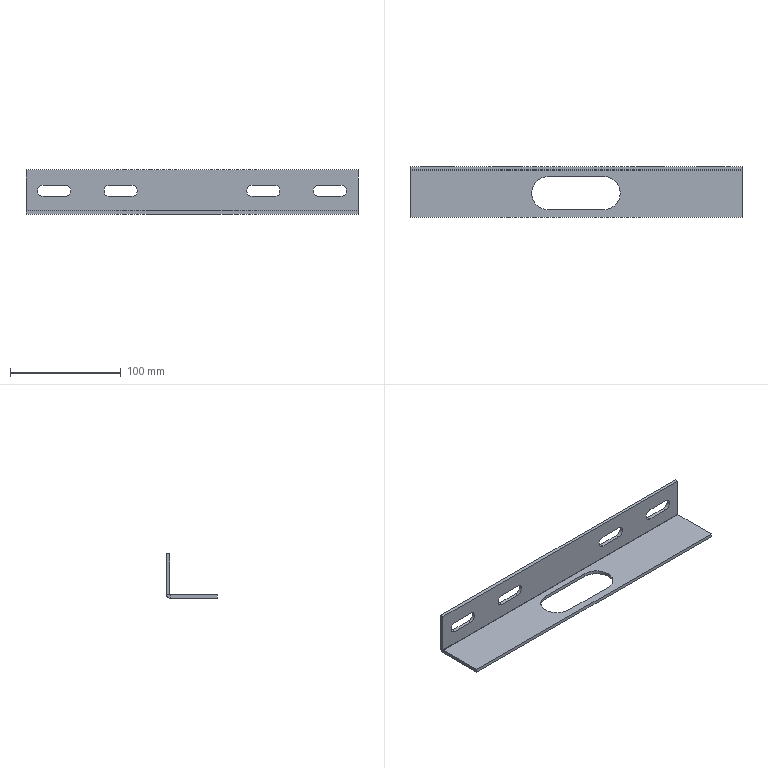Part | 1 solid | 35 faces | box 300 x 46 x 40 mm | volume 64080 mm3 | plane 22 | cylinder 13 | commonest cylinder face diameters 10 x8 30 x3 0.4 x1 6.4 x1
STEP:
#1=CARTESIAN_POINT('',(40.,-1.,-3.));
#2=VERTEX_POINT('',#1);
#3=CARTESIAN_POINT('',(25.,14.,-3.));
#4=VERTEX_POINT('',#3);
#5=CARTESIAN_POINT('',(25.,-1.,-3.));
#6=DIRECTION('',(0.,0.,1.));
#7=DIRECTION('',(1.,0.,0.));
#8=AXIS2_PLACEMENT_3D('',#5,#6,#7);
#9=CIRCLE('',#8,15.);
#10=EDGE_CURVE('',#2,#4,#9,.T.);
#11=ORIENTED_EDGE('',*,*,#10,.F.);
#12=CARTESIAN_POINT('',(40.,-1.,0.));
#13=VERTEX_POINT('',#12);
#14=CARTESIAN_POINT('',(40.,-1.,-10.));
#15=DIRECTION('',(0.,0.,1.));
#16=VECTOR('',#15,1000.);
#17=LINE('',#14,#16);
#18=EDGE_CURVE('',#2,#13,#17,.T.);
#19=ORIENTED_EDGE('',*,*,#18,.T.);
#20=CARTESIAN_POINT('',(25.,14.,0.));
#21=VERTEX_POINT('',#20);
#22=CARTESIAN_POINT('',(25.,-1.,0.));
#23=DIRECTION('',(0.,0.,1.));
#24=DIRECTION('',(1.,0.,0.));
#25=AXIS2_PLACEMENT_3D('',#22,#23,#24);
#26=CIRCLE('',#25,15.);
#27=EDGE_CURVE('',#13,#21,#26,.T.);
#28=ORIENTED_EDGE('',*,*,#27,.T.);
#29=CARTESIAN_POINT('',(25.,14.,-10.));
#30=DIRECTION('',(0.,0.,1.));
#31=VECTOR('',#30,1000.);
#32=LINE('',#29,#31);
#33=EDGE_CURVE('',#4,#21,#32,.T.);
#34=ORIENTED_EDGE('',*,*,#33,.F.);
#35=EDGE_LOOP('',(#11,#19,#28,#34));
#36=FACE_OUTER_BOUND('',#35,.T.);
#37=CARTESIAN_POINT('',(25.,-1.,-10.));
#38=DIRECTION('',(0.,0.,1.));
#39=DIRECTION('',(1.,0.,0.));
#40=AXIS2_PLACEMENT_3D('',#37,#38,#39);
#41=CYLINDRICAL_SURFACE('',#40,15.);
#42=ADVANCED_FACE('',(#36),#41,.F.);
#43=CARTESIAN_POINT('',(-150.,19.8,0.));
#44=VERTEX_POINT('',#43);
#45=CARTESIAN_POINT('',(-150.,-23.,0.));
#46=VERTEX_POINT('',#45);
#47=CARTESIAN_POINT('',(-150.,23.,0.));
#48=DIRECTION('',(0.,-1.,0.));
#49=VECTOR('',#48,1000.);
#50=LINE('',#47,#49);
#51=EDGE_CURVE('',#44,#46,#50,.T.);
#52=ORIENTED_EDGE('',*,*,#51,.F.);
#53=CARTESIAN_POINT('',(-150.,19.8,-3.));
#54=VERTEX_POINT('',#53);
#55=CARTESIAN_POINT('',(-150.,19.8,0.));
#56=DIRECTION('',(0.,0.,-1.));
#57=VECTOR('',#56,1000.);
#58=LINE('',#55,#57);
#59=EDGE_CURVE('',#44,#54,#58,.T.);
#60=ORIENTED_EDGE('',*,*,#59,.T.);
#61=CARTESIAN_POINT('',(-150.,-23.,-3.));
#62=VERTEX_POINT('',#61);
#63=CARTESIAN_POINT('',(-150.,23.,-3.));
#64=DIRECTION('',(0.,-1.,0.));
#65=VECTOR('',#64,1000.);
#66=LINE('',#63,#65);
#67=EDGE_CURVE('',#54,#62,#66,.T.);
#68=ORIENTED_EDGE('',*,*,#67,.T.);
#69=CARTESIAN_POINT('',(-150.,-23.,-3.));
#70=DIRECTION('',(0.,0.,1.));
#71=VECTOR('',#70,1000.);
#72=LINE('',#69,#71);
#73=EDGE_CURVE('',#62,#46,#72,.T.);
#74=ORIENTED_EDGE('',*,*,#73,.T.);
#75=EDGE_LOOP('',(#52,#60,#68,#74));
#76=FACE_OUTER_BOUND('',#75,.T.);
#77=CARTESIAN_POINT('',(-150.,23.,-3.));
#78=DIRECTION('',(-1.,0.,0.));
#79=DIRECTION('',(0.,0.,1.));
#80=AXIS2_PLACEMENT_3D('',#77,#78,#79);
#81=PLANE('',#80);
#82=ADVANCED_FACE('',(#76),#81,.T.);
#83=CARTESIAN_POINT('',(-25.,14.,-3.));
#84=VERTEX_POINT('',#83);
#85=CARTESIAN_POINT('',(0.,14.,-3.));
#86=DIRECTION('',(-1.,0.,0.));
#87=VECTOR('',#86,1000.);
#88=LINE('',#85,#87);
#89=EDGE_CURVE('',#4,#84,#88,.T.);
#90=ORIENTED_EDGE('',*,*,#89,.T.);
#91=CARTESIAN_POINT('',(-25.,-16.,-3.));
#92=VERTEX_POINT('',#91);
#93=CARTESIAN_POINT('',(-25.,-1.,-3.));
#94=DIRECTION('',(0.,0.,1.));
#95=DIRECTION('',(1.,0.,0.));
#96=AXIS2_PLACEMENT_3D('',#93,#94,#95);
#97=CIRCLE('',#96,15.);
#98=EDGE_CURVE('',#84,#92,#97,.T.);
#99=ORIENTED_EDGE('',*,*,#98,.T.);
#100=CARTESIAN_POINT('',(25.,-16.,-3.));
#101=VERTEX_POINT('',#100);
#102=CARTESIAN_POINT('',(0.,-16.,-3.));
#103=DIRECTION('',(1.,0.,0.));
#104=VECTOR('',#103,1000.);
#105=LINE('',#102,#104);
#106=EDGE_CURVE('',#92,#101,#105,.T.);
#107=ORIENTED_EDGE('',*,*,#106,.T.);
#108=CARTESIAN_POINT('',(25.,-1.,-3.));
#109=DIRECTION('',(0.,0.,1.));
#110=DIRECTION('',(1.,0.,0.));
#111=AXIS2_PLACEMENT_3D('',#108,#109,#110);
#112=CIRCLE('',#111,15.);
#113=EDGE_CURVE('',#101,#2,#112,.T.);
#114=ORIENTED_EDGE('',*,*,#113,.T.);
#115=ORIENTED_EDGE('',*,*,#10,.T.);
#116=EDGE_LOOP('',(#90,#99,#107,#114,#115));
#117=FACE_BOUND('',#116,.T.);
#118=CARTESIAN_POINT('',(150.,19.8,-3.));
#119=VERTEX_POINT('',#118);
#120=CARTESIAN_POINT('',(-150.,19.8,-3.));
#121=DIRECTION('',(1.,0.,0.));
#122=VECTOR('',#121,1000.);
#123=LINE('',#120,#122);
#124=EDGE_CURVE('',#54,#119,#123,.T.);
#125=ORIENTED_EDGE('',*,*,#124,.T.);
#126=CARTESIAN_POINT('',(150.,-23.,-3.));
#127=VERTEX_POINT('',#126);
#128=CARTESIAN_POINT('',(150.,23.,-3.));
#129=DIRECTION('',(0.,1.,0.));
#130=VECTOR('',#129,1000.);
#131=LINE('',#128,#130);
#132=EDGE_CURVE('',#127,#119,#131,.T.);
#133=ORIENTED_EDGE('',*,*,#132,.F.);
#134=CARTESIAN_POINT('',(-150.,-23.,-3.));
#135=DIRECTION('',(1.,0.,0.));
#136=VECTOR('',#135,1000.);
#137=LINE('',#134,#136);
#138=EDGE_CURVE('',#62,#127,#137,.T.);
#139=ORIENTED_EDGE('',*,*,#138,.F.);
#140=ORIENTED_EDGE('',*,*,#67,.F.);
#141=EDGE_LOOP('',(#125,#133,#139,#140));
#142=FACE_OUTER_BOUND('',#141,.T.);
#143=CARTESIAN_POINT('',(0.,0.,-3.));
#144=DIRECTION('',(0.,0.,1.));
#145=DIRECTION('',(1.,0.,0.));
#146=AXIS2_PLACEMENT_3D('',#143,#144,#145);
#147=PLANE('',#146);
#148=ADVANCED_FACE('',(#117,#142),#147,.F.);
#149=CARTESIAN_POINT('',(-25.,14.,0.));
#150=VERTEX_POINT('',#149);
#151=CARTESIAN_POINT('',(-25.,-16.,0.));
#152=VERTEX_POINT('',#151);
#153=CARTESIAN_POINT('',(-25.,-1.,0.));
#154=DIRECTION('',(0.,0.,1.));
#155=DIRECTION('',(1.,0.,0.));
#156=AXIS2_PLACEMENT_3D('',#153,#154,#155);
#157=CIRCLE('',#156,15.);
#158=EDGE_CURVE('',#150,#152,#157,.T.);
#159=ORIENTED_EDGE('',*,*,#158,.F.);
#160=CARTESIAN_POINT('',(-25.,14.,0.));
#161=DIRECTION('',(-1.,0.,0.));
#162=VECTOR('',#161,1000.);
#163=LINE('',#160,#162);
#164=EDGE_CURVE('',#21,#150,#163,.T.);
#165=ORIENTED_EDGE('',*,*,#164,.F.);
#166=ORIENTED_EDGE('',*,*,#27,.F.);
#167=CARTESIAN_POINT('',(25.,-16.,0.));
#168=VERTEX_POINT('',#167);
#169=CARTESIAN_POINT('',(25.,-1.,0.));
#170=DIRECTION('',(0.,0.,1.));
#171=DIRECTION('',(1.,0.,0.));
#172=AXIS2_PLACEMENT_3D('',#169,#170,#171);
#173=CIRCLE('',#172,15.);
#174=EDGE_CURVE('',#168,#13,#173,.T.);
#175=ORIENTED_EDGE('',*,*,#174,.F.);
#176=CARTESIAN_POINT('',(-25.,-16.,0.));
#177=DIRECTION('',(1.,0.,0.));
#178=VECTOR('',#177,1000.);
#179=LINE('',#176,#178);
#180=EDGE_CURVE('',#152,#168,#179,.T.);
#181=ORIENTED_EDGE('',*,*,#180,.F.);
#182=EDGE_LOOP('',(#159,#165,#166,#175,#181));
#183=FACE_BOUND('',#182,.T.);
#184=CARTESIAN_POINT('',(150.,-23.,0.));
#185=VERTEX_POINT('',#184);
#186=CARTESIAN_POINT('',(150.,19.8,0.));
#187=VERTEX_POINT('',#186);
#188=CARTESIAN_POINT('',(150.,23.,0.));
#189=DIRECTION('',(0.,1.,0.));
#190=VECTOR('',#189,1000.);
#191=LINE('',#188,#190);
#192=EDGE_CURVE('',#185,#187,#191,.T.);
#193=ORIENTED_EDGE('',*,*,#192,.T.);
#194=CARTESIAN_POINT('',(-150.,19.8,0.));
#195=DIRECTION('',(1.,0.,0.));
#196=VECTOR('',#195,1000.);
#197=LINE('',#194,#196);
#198=EDGE_CURVE('',#44,#187,#197,.T.);
#199=ORIENTED_EDGE('',*,*,#198,.F.);
#200=ORIENTED_EDGE('',*,*,#51,.T.);
#201=CARTESIAN_POINT('',(-150.,-23.,0.));
#202=DIRECTION('',(1.,0.,0.));
#203=VECTOR('',#202,1000.);
#204=LINE('',#201,#203);
#205=EDGE_CURVE('',#46,#185,#204,.T.);
#206=ORIENTED_EDGE('',*,*,#205,.T.);
#207=EDGE_LOOP('',(#193,#199,#200,#206));
#208=FACE_OUTER_BOUND('',#207,.T.);
#209=CARTESIAN_POINT('',(0.,0.,0.));
#210=DIRECTION('',(0.,0.,1.));
#211=DIRECTION('',(1.,0.,0.));
#212=AXIS2_PLACEMENT_3D('',#209,#210,#211);
#213=PLANE('',#212);
#214=ADVANCED_FACE('',(#183,#208),#213,.T.);
#215=CARTESIAN_POINT('',(150.,19.8,0.));
#216=DIRECTION('',(0.,0.,-1.));
#217=VECTOR('',#216,1000.);
#218=LINE('',#215,#217);
#219=EDGE_CURVE('',#187,#119,#218,.T.);
#220=ORIENTED_EDGE('',*,*,#219,.F.);
#221=ORIENTED_EDGE('',*,*,#192,.F.);
#222=CARTESIAN_POINT('',(150.,-23.,-3.));
#223=DIRECTION('',(0.,0.,1.));
#224=VECTOR('',#223,1000.);
#225=LINE('',#222,#224);
#226=EDGE_CURVE('',#127,#185,#225,.T.);
#227=ORIENTED_EDGE('',*,*,#226,.F.);
#228=ORIENTED_EDGE('',*,*,#132,.T.);
#229=EDGE_LOOP('',(#220,#221,#227,#228));
#230=FACE_OUTER_BOUND('',#229,.T.);
#231=CARTESIAN_POINT('',(150.,23.,-3.));
#232=DIRECTION('',(1.,0.,0.));
#233=DIRECTION('',(0.,0.,-1.));
#234=AXIS2_PLACEMENT_3D('',#231,#232,#233);
#235=PLANE('',#234);
#236=ADVANCED_FACE('',(#230),#235,.T.);
#237=ORIENTED_EDGE('',*,*,#205,.F.);
#238=ORIENTED_EDGE('',*,*,#73,.F.);
#239=ORIENTED_EDGE('',*,*,#138,.T.);
#240=ORIENTED_EDGE('',*,*,#226,.T.);
#241=EDGE_LOOP('',(#237,#238,#239,#240));
#242=FACE_OUTER_BOUND('',#241,.T.);
#243=CARTESIAN_POINT('',(-150.,-23.,-3.));
#244=DIRECTION('',(0.,-1.,0.));
#245=DIRECTION('',(0.,0.,-1.));
#246=AXIS2_PLACEMENT_3D('',#243,#244,#245);
#247=PLANE('',#246);
#248=ADVANCED_FACE('',(#242),#247,.T.);
#249=CARTESIAN_POINT('',(150.,20.,0.2));
#250=VERTEX_POINT('',#249);
#251=CARTESIAN_POINT('',(150.,23.,0.2));
#252=VERTEX_POINT('',#251);
#253=CARTESIAN_POINT('',(150.,23.,0.2));
#254=DIRECTION('',(0.,1.,0.));
#255=VECTOR('',#254,1000.);
#256=LINE('',#253,#255);
#257=EDGE_CURVE('',#250,#252,#256,.T.);
#258=ORIENTED_EDGE('',*,*,#257,.F.);
#259=CARTESIAN_POINT('',(150.,19.8,0.2));
#260=DIRECTION('',(1.,0.,0.));
#261=DIRECTION('',(0.,0.,1.));
#262=AXIS2_PLACEMENT_3D('',#259,#260,#261);
#263=CIRCLE('',#262,0.2);
#264=EDGE_CURVE('',#187,#250,#263,.T.);
#265=ORIENTED_EDGE('',*,*,#264,.F.);
#266=ORIENTED_EDGE('',*,*,#219,.T.);
#267=CARTESIAN_POINT('',(150.,19.8,0.2));
#268=DIRECTION('',(1.,0.,0.));
#269=DIRECTION('',(0.,0.,1.));
#270=AXIS2_PLACEMENT_3D('',#267,#268,#269);
#271=CIRCLE('',#270,3.2);
#272=EDGE_CURVE('',#119,#252,#271,.T.);
#273=ORIENTED_EDGE('',*,*,#272,.T.);
#274=EDGE_LOOP('',(#258,#265,#266,#273));
#275=FACE_OUTER_BOUND('',#274,.T.);
#276=CARTESIAN_POINT('',(150.,19.8,0.2));
#277=DIRECTION('',(1.,0.,0.));
#278=DIRECTION('',(0.,0.,-1.));
#279=AXIS2_PLACEMENT_3D('',#276,#277,#278);
#280=PLANE('',#279);
#281=ADVANCED_FACE('',(#275),#280,.T.);
#282=CARTESIAN_POINT('',(-150.,20.,0.2));
#283=VERTEX_POINT('',#282);
#284=CARTESIAN_POINT('',(-150.,19.8,0.2));
#285=DIRECTION('',(-1.,0.,0.));
#286=DIRECTION('',(0.,0.,1.));
#287=AXIS2_PLACEMENT_3D('',#284,#285,#286);
#288=CIRCLE('',#287,0.2);
#289=EDGE_CURVE('',#283,#44,#288,.T.);
#290=ORIENTED_EDGE('',*,*,#289,.F.);
#291=CARTESIAN_POINT('',(-150.,23.,0.2));
#292=VERTEX_POINT('',#291);
#293=CARTESIAN_POINT('',(-150.,20.,0.2));
#294=DIRECTION('',(0.,1.,0.));
#295=VECTOR('',#294,1000.);
#296=LINE('',#293,#295);
#297=EDGE_CURVE('',#283,#292,#296,.T.);
#298=ORIENTED_EDGE('',*,*,#297,.T.);
#299=CARTESIAN_POINT('',(-150.,19.8,0.2));
#300=DIRECTION('',(-1.,0.,0.));
#301=DIRECTION('',(0.,0.,1.));
#302=AXIS2_PLACEMENT_3D('',#299,#300,#301);
#303=CIRCLE('',#302,3.2);
#304=EDGE_CURVE('',#292,#54,#303,.T.);
#305=ORIENTED_EDGE('',*,*,#304,.T.);
#306=ORIENTED_EDGE('',*,*,#59,.F.);
#307=EDGE_LOOP('',(#290,#298,#305,#306));
#308=FACE_OUTER_BOUND('',#307,.T.);
#309=CARTESIAN_POINT('',(-150.,19.8,0.2));
#310=DIRECTION('',(1.,0.,0.));
#311=DIRECTION('',(0.,0.,-1.));
#312=AXIS2_PLACEMENT_3D('',#309,#310,#311);
#313=PLANE('',#312);
#314=ADVANCED_FACE('',(#308),#313,.F.);
#315=ORIENTED_EDGE('',*,*,#124,.F.);
#316=ORIENTED_EDGE('',*,*,#304,.F.);
#317=CARTESIAN_POINT('',(150.,23.,0.2));
#318=DIRECTION('',(1.,0.,0.));
#319=VECTOR('',#318,1000.);
#320=LINE('',#317,#319);
#321=EDGE_CURVE('',#292,#252,#320,.T.);
#322=ORIENTED_EDGE('',*,*,#321,.T.);
#323=ORIENTED_EDGE('',*,*,#272,.F.);
#324=EDGE_LOOP('',(#315,#316,#322,#323));
#325=FACE_OUTER_BOUND('',#324,.T.);
#326=CARTESIAN_POINT('',(-150.,19.8,0.2));
#327=DIRECTION('',(-1.,0.,0.));
#328=DIRECTION('',(0.,1.,0.));
#329=AXIS2_PLACEMENT_3D('',#326,#327,#328);
#330=CYLINDRICAL_SURFACE('',#329,3.2);
#331=ADVANCED_FACE('',(#325),#330,.T.);
#332=ORIENTED_EDGE('',*,*,#198,.T.);
#333=ORIENTED_EDGE('',*,*,#264,.T.);
#334=CARTESIAN_POINT('',(150.,20.,0.2));
#335=DIRECTION('',(-1.,0.,0.));
#336=VECTOR('',#335,1000.);
#337=LINE('',#334,#336);
#338=EDGE_CURVE('',#250,#283,#337,.T.);
#339=ORIENTED_EDGE('',*,*,#338,.T.);
#340=ORIENTED_EDGE('',*,*,#289,.T.);
#341=EDGE_LOOP('',(#332,#333,#339,#340));
#342=FACE_OUTER_BOUND('',#341,.T.);
#343=CARTESIAN_POINT('',(-150.,19.8,0.2));
#344=DIRECTION('',(-1.,0.,0.));
#345=DIRECTION('',(0.,1.,0.));
#346=AXIS2_PLACEMENT_3D('',#343,#344,#345);
#347=CYLINDRICAL_SURFACE('',#346,0.2);
#348=ADVANCED_FACE('',(#342),#347,.F.);
#349=ORIENTED_EDGE('',*,*,#257,.T.);
#350=CARTESIAN_POINT('',(150.,23.,37.));
#351=VERTEX_POINT('',#350);
#352=CARTESIAN_POINT('',(150.,23.,0.));
#353=DIRECTION('',(0.,0.,-1.));
#354=VECTOR('',#353,1000.);
#355=LINE('',#352,#354);
#356=EDGE_CURVE('',#351,#252,#355,.T.);
#357=ORIENTED_EDGE('',*,*,#356,.F.);
#358=CARTESIAN_POINT('',(150.,20.,37.));
#359=VERTEX_POINT('',#358);
#360=CARTESIAN_POINT('',(150.,23.,37.));
#361=DIRECTION('',(0.,-1.,0.));
#362=VECTOR('',#361,1000.);
#363=LINE('',#360,#362);
#364=EDGE_CURVE('',#351,#359,#363,.T.);
#365=ORIENTED_EDGE('',*,*,#364,.T.);
#366=CARTESIAN_POINT('',(150.,20.,0.));
#367=DIRECTION('',(0.,0.,-1.));
#368=VECTOR('',#367,1000.);
#369=LINE('',#366,#368);
#370=EDGE_CURVE('',#359,#250,#369,.T.);
#371=ORIENTED_EDGE('',*,*,#370,.T.);
#372=EDGE_LOOP('',(#349,#357,#365,#371));
#373=FACE_OUTER_BOUND('',#372,.T.);
#374=CARTESIAN_POINT('',(150.,23.,0.));
#375=DIRECTION('',(-1.,0.,0.));
#376=DIRECTION('',(0.,0.,1.));
#377=AXIS2_PLACEMENT_3D('',#374,#375,#376);
#378=PLANE('',#377);
#379=ADVANCED_FACE('',(#373),#378,.F.);
#380=ORIENTED_EDGE('',*,*,#297,.F.);
#381=CARTESIAN_POINT('',(-150.,20.,37.));
#382=VERTEX_POINT('',#381);
#383=CARTESIAN_POINT('',(-150.,20.,37.));
#384=DIRECTION('',(0.,0.,1.));
#385=VECTOR('',#384,1000.);
#386=LINE('',#383,#385);
#387=EDGE_CURVE('',#283,#382,#386,.T.);
#388=ORIENTED_EDGE('',*,*,#387,.T.);
#389=CARTESIAN_POINT('',(-150.,23.,37.));
#390=VERTEX_POINT('',#389);
#391=CARTESIAN_POINT('',(-150.,23.,37.));
#392=DIRECTION('',(0.,-1.,0.));
#393=VECTOR('',#392,1000.);
#394=LINE('',#391,#393);
#395=EDGE_CURVE('',#390,#382,#394,.T.);
#396=ORIENTED_EDGE('',*,*,#395,.F.);
#397=CARTESIAN_POINT('',(-150.,23.,0.));
#398=DIRECTION('',(0.,0.,1.));
#399=VECTOR('',#398,1000.);
#400=LINE('',#397,#399);
#401=EDGE_CURVE('',#292,#390,#400,.T.);
#402=ORIENTED_EDGE('',*,*,#401,.F.);
#403=EDGE_LOOP('',(#380,#388,#396,#402));
#404=FACE_OUTER_BOUND('',#403,.T.);
#405=CARTESIAN_POINT('',(-150.,23.,37.));
#406=DIRECTION('',(1.,0.,0.));
#407=DIRECTION('',(0.,0.,-1.));
#408=AXIS2_PLACEMENT_3D('',#405,#406,#407);
#409=PLANE('',#408);
#410=ADVANCED_FACE('',(#404),#409,.F.);
#411=CARTESIAN_POINT('',(-134.5,23.,23.));
#412=VERTEX_POINT('',#411);
#413=CARTESIAN_POINT('',(-114.5,23.,23.));
#414=VERTEX_POINT('',#413);
#415=CARTESIAN_POINT('',(-134.5,23.,23.));
#416=DIRECTION('',(1.,0.,0.));
#417=VECTOR('',#416,1000.);
#418=LINE('',#415,#417);
#419=EDGE_CURVE('',#412,#414,#418,.T.);
#420=ORIENTED_EDGE('',*,*,#419,.F.);
#421=CARTESIAN_POINT('',(-134.5,23.,13.));
#422=VERTEX_POINT('',#421);
#423=CARTESIAN_POINT('',(-134.5,23.,18.));
#424=DIRECTION('',(0.,1.,0.));
#425=DIRECTION('',(0.,0.,1.));
#426=AXIS2_PLACEMENT_3D('',#423,#424,#425);
#427=CIRCLE('',#426,5.);
#428=EDGE_CURVE('',#422,#412,#427,.T.);
#429=ORIENTED_EDGE('',*,*,#428,.F.);
#430=CARTESIAN_POINT('',(-114.5,23.,13.));
#431=VERTEX_POINT('',#430);
#432=CARTESIAN_POINT('',(-134.5,23.,13.));
#433=DIRECTION('',(-1.,0.,0.));
#434=VECTOR('',#433,1000.);
#435=LINE('',#432,#434);
#436=EDGE_CURVE('',#431,#422,#435,.T.);
#437=ORIENTED_EDGE('',*,*,#436,.F.);
#438=CARTESIAN_POINT('',(-114.5,23.,18.));
#439=DIRECTION('',(0.,1.,0.));
#440=DIRECTION('',(0.,0.,1.));
#441=AXIS2_PLACEMENT_3D('',#438,#439,#440);
#442=CIRCLE('',#441,5.);
#443=EDGE_CURVE('',#414,#431,#442,.T.);
#444=ORIENTED_EDGE('',*,*,#443,.F.);
#445=EDGE_LOOP('',(#420,#429,#437,#444));
#446=FACE_BOUND('',#445,.T.);
#447=CARTESIAN_POINT('',(-74.5,23.,23.));
#448=VERTEX_POINT('',#447);
#449=CARTESIAN_POINT('',(-54.5,23.,23.));
#450=VERTEX_POINT('',#449);
#451=CARTESIAN_POINT('',(-74.5,23.,23.));
#452=DIRECTION('',(1.,0.,0.));
#453=VECTOR('',#452,1000.);
#454=LINE('',#451,#453);
#455=EDGE_CURVE('',#448,#450,#454,.T.);
#456=ORIENTED_EDGE('',*,*,#455,.F.);
#457=CARTESIAN_POINT('',(-74.5,23.,13.));
#458=VERTEX_POINT('',#457);
#459=CARTESIAN_POINT('',(-74.5,23.,18.));
#460=DIRECTION('',(0.,1.,0.));
#461=DIRECTION('',(0.,0.,1.));
#462=AXIS2_PLACEMENT_3D('',#459,#460,#461);
#463=CIRCLE('',#462,5.);
#464=EDGE_CURVE('',#458,#448,#463,.T.);
#465=ORIENTED_EDGE('',*,*,#464,.F.);
#466=CARTESIAN_POINT('',(-54.5,23.,13.));
#467=VERTEX_POINT('',#466);
#468=CARTESIAN_POINT('',(-74.5,23.,13.));
#469=DIRECTION('',(-1.,0.,0.));
#470=VECTOR('',#469,1000.);
#471=LINE('',#468,#470);
#472=EDGE_CURVE('',#467,#458,#471,.T.);
#473=ORIENTED_EDGE('',*,*,#472,.F.);
#474=CARTESIAN_POINT('',(-54.5,23.,18.));
#475=DIRECTION('',(0.,1.,0.));
#476=DIRECTION('',(0.,0.,1.));
#477=AXIS2_PLACEMENT_3D('',#474,#475,#476);
#478=CIRCLE('',#477,5.);
#479=EDGE_CURVE('',#450,#467,#478,.T.);
#480=ORIENTED_EDGE('',*,*,#479,.F.);
#481=EDGE_LOOP('',(#456,#465,#473,#480));
#482=FACE_BOUND('',#481,.T.);
#483=CARTESIAN_POINT('',(74.5,23.,13.));
#484=VERTEX_POINT('',#483);
#485=CARTESIAN_POINT('',(54.5,23.,13.));
#486=VERTEX_POINT('',#485);
#487=CARTESIAN_POINT('',(74.5,23.,13.));
#488=DIRECTION('',(-1.,0.,0.));
#489=VECTOR('',#488,1000.);
#490=LINE('',#487,#489);
#491=EDGE_CURVE('',#484,#486,#490,.T.);
#492=ORIENTED_EDGE('',*,*,#491,.F.);
#493=CARTESIAN_POINT('',(74.5,23.,23.));
#494=VERTEX_POINT('',#493);
#495=CARTESIAN_POINT('',(74.5,23.,18.));
#496=DIRECTION('',(0.,1.,0.));
#497=DIRECTION('',(0.,0.,-1.));
#498=AXIS2_PLACEMENT_3D('',#495,#496,#497);
#499=CIRCLE('',#498,5.);
#500=EDGE_CURVE('',#494,#484,#499,.T.);
#501=ORIENTED_EDGE('',*,*,#500,.F.);
#502=CARTESIAN_POINT('',(54.5,23.,23.));
#503=VERTEX_POINT('',#502);
#504=CARTESIAN_POINT('',(74.5,23.,23.));
#505=DIRECTION('',(1.,0.,0.));
#506=VECTOR('',#505,1000.);
#507=LINE('',#504,#506);
#508=EDGE_CURVE('',#503,#494,#507,.T.);
#509=ORIENTED_EDGE('',*,*,#508,.F.);
#510=CARTESIAN_POINT('',(54.5,23.,18.));
#511=DIRECTION('',(0.,1.,0.));
#512=DIRECTION('',(0.,0.,-1.));
#513=AXIS2_PLACEMENT_3D('',#510,#511,#512);
#514=CIRCLE('',#513,5.);
#515=EDGE_CURVE('',#486,#503,#514,.T.);
#516=ORIENTED_EDGE('',*,*,#515,.F.);
#517=EDGE_LOOP('',(#492,#501,#509,#516));
#518=FACE_BOUND('',#517,.T.);
#519=CARTESIAN_POINT('',(134.5,23.,13.));
#520=VERTEX_POINT('',#519);
#521=CARTESIAN_POINT('',(114.5,23.,13.));
#522=VERTEX_POINT('',#521);
#523=CARTESIAN_POINT('',(134.5,23.,13.));
#524=DIRECTION('',(-1.,0.,0.));
#525=VECTOR('',#524,1000.);
#526=LINE('',#523,#525);
#527=EDGE_CURVE('',#520,#522,#526,.T.);
#528=ORIENTED_EDGE('',*,*,#527,.F.);
#529=CARTESIAN_POINT('',(134.5,23.,23.));
#530=VERTEX_POINT('',#529);
#531=CARTESIAN_POINT('',(134.5,23.,18.));
#532=DIRECTION('',(0.,1.,0.));
#533=DIRECTION('',(0.,0.,-1.));
#534=AXIS2_PLACEMENT_3D('',#531,#532,#533);
#535=CIRCLE('',#534,5.);
#536=EDGE_CURVE('',#530,#520,#535,.T.);
#537=ORIENTED_EDGE('',*,*,#536,.F.);
#538=CARTESIAN_POINT('',(114.5,23.,23.));
#539=VERTEX_POINT('',#538);
#540=CARTESIAN_POINT('',(134.5,23.,23.));
#541=DIRECTION('',(1.,0.,0.));
#542=VECTOR('',#541,1000.);
#543=LINE('',#540,#542);
#544=EDGE_CURVE('',#539,#530,#543,.T.);
#545=ORIENTED_EDGE('',*,*,#544,.F.);
#546=CARTESIAN_POINT('',(114.5,23.,18.));
#547=DIRECTION('',(0.,1.,0.));
#548=DIRECTION('',(0.,0.,-1.));
#549=AXIS2_PLACEMENT_3D('',#546,#547,#548);
#550=CIRCLE('',#549,5.);
#551=EDGE_CURVE('',#522,#539,#550,.T.);
#552=ORIENTED_EDGE('',*,*,#551,.F.);
#553=EDGE_LOOP('',(#528,#537,#545,#552));
#554=FACE_BOUND('',#553,.T.);
#555=ORIENTED_EDGE('',*,*,#321,.F.);
#556=ORIENTED_EDGE('',*,*,#401,.T.);
#557=CARTESIAN_POINT('',(0.,23.,37.));
#558=DIRECTION('',(1.,0.,0.));
#559=VECTOR('',#558,1000.);
#560=LINE('',#557,#559);
#561=EDGE_CURVE('',#390,#351,#560,.T.);
#562=ORIENTED_EDGE('',*,*,#561,.T.);
#563=ORIENTED_EDGE('',*,*,#356,.T.);
#564=EDGE_LOOP('',(#555,#556,#562,#563));
#565=FACE_OUTER_BOUND('',#564,.T.);
#566=CARTESIAN_POINT('',(0.,23.,0.));
#567=DIRECTION('',(0.,-1.,0.));
#568=DIRECTION('',(0.,0.,-1.));
#569=AXIS2_PLACEMENT_3D('',#566,#567,#568);
#570=PLANE('',#569);
#571=ADVANCED_FACE('',(#446,#482,#518,#554,#565),#570,.F.);
#572=CARTESIAN_POINT('',(-134.5,20.,23.));
#573=VERTEX_POINT('',#572);
#574=CARTESIAN_POINT('',(-134.5,20.,13.));
#575=VERTEX_POINT('',#574);
#576=CARTESIAN_POINT('',(-134.5,20.,18.));
#577=DIRECTION('',(0.,-1.,0.));
#578=DIRECTION('',(0.,0.,-1.));
#579=AXIS2_PLACEMENT_3D('',#576,#577,#578);
#580=CIRCLE('',#579,5.);
#581=EDGE_CURVE('',#573,#575,#580,.T.);
#582=ORIENTED_EDGE('',*,*,#581,.F.);
#583=CARTESIAN_POINT('',(-114.5,20.,23.));
#584=VERTEX_POINT('',#583);
#585=CARTESIAN_POINT('',(0.,20.,23.));
#586=DIRECTION('',(-1.,0.,0.));
#587=VECTOR('',#586,1000.);
#588=LINE('',#585,#587);
#589=EDGE_CURVE('',#584,#573,#588,.T.);
#590=ORIENTED_EDGE('',*,*,#589,.F.);
#591=CARTESIAN_POINT('',(-114.5,20.,13.));
#592=VERTEX_POINT('',#591);
#593=CARTESIAN_POINT('',(-114.5,20.,18.));
#594=DIRECTION('',(0.,-1.,0.));
#595=DIRECTION('',(0.,0.,-1.));
#596=AXIS2_PLACEMENT_3D('',#593,#594,#595);
#597=CIRCLE('',#596,5.);
#598=EDGE_CURVE('',#592,#584,#597,.T.);
#599=ORIENTED_EDGE('',*,*,#598,.F.);
#600=CARTESIAN_POINT('',(0.,20.,13.));
#601=DIRECTION('',(1.,0.,0.));
#602=VECTOR('',#601,1000.);
#603=LINE('',#600,#602);
#604=EDGE_CURVE('',#575,#592,#603,.T.);
#605=ORIENTED_EDGE('',*,*,#604,.F.);
#606=EDGE_LOOP('',(#582,#590,#599,#605));
#607=FACE_BOUND('',#606,.T.);
#608=CARTESIAN_POINT('',(-74.5,20.,23.));
#609=VERTEX_POINT('',#608);
#610=CARTESIAN_POINT('',(-74.5,20.,13.));
#611=VERTEX_POINT('',#610);
#612=CARTESIAN_POINT('',(-74.5,20.,18.));
#613=DIRECTION('',(0.,-1.,0.));
#614=DIRECTION('',(0.,0.,-1.));
#615=AXIS2_PLACEMENT_3D('',#612,#613,#614);
#616=CIRCLE('',#615,5.);
#617=EDGE_CURVE('',#609,#611,#616,.T.);
#618=ORIENTED_EDGE('',*,*,#617,.F.);
#619=CARTESIAN_POINT('',(-54.5,20.,23.));
#620=VERTEX_POINT('',#619);
#621=CARTESIAN_POINT('',(0.,20.,23.));
#622=DIRECTION('',(-1.,0.,0.));
#623=VECTOR('',#622,1000.);
#624=LINE('',#621,#623);
#625=EDGE_CURVE('',#620,#609,#624,.T.);
#626=ORIENTED_EDGE('',*,*,#625,.F.);
#627=CARTESIAN_POINT('',(-54.5,20.,13.));
#628=VERTEX_POINT('',#627);
#629=CARTESIAN_POINT('',(-54.5,20.,18.));
#630=DIRECTION('',(0.,-1.,0.));
#631=DIRECTION('',(0.,0.,-1.));
#632=AXIS2_PLACEMENT_3D('',#629,#630,#631);
#633=CIRCLE('',#632,5.);
#634=EDGE_CURVE('',#628,#620,#633,.T.);
#635=ORIENTED_EDGE('',*,*,#634,.F.);
#636=CARTESIAN_POINT('',(0.,20.,13.));
#637=DIRECTION('',(1.,0.,0.));
#638=VECTOR('',#637,1000.);
#639=LINE('',#636,#638);
#640=EDGE_CURVE('',#611,#628,#639,.T.);
#641=ORIENTED_EDGE('',*,*,#640,.F.);
#642=EDGE_LOOP('',(#618,#626,#635,#641));
#643=FACE_BOUND('',#642,.T.);
#644=CARTESIAN_POINT('',(74.5,20.,13.));
#645=VERTEX_POINT('',#644);
#646=CARTESIAN_POINT('',(74.5,20.,23.));
#647=VERTEX_POINT('',#646);
#648=CARTESIAN_POINT('',(74.5,20.,18.));
#649=DIRECTION('',(0.,-1.,0.));
#650=DIRECTION('',(0.,0.,-1.));
#651=AXIS2_PLACEMENT_3D('',#648,#649,#650);
#652=CIRCLE('',#651,5.);
#653=EDGE_CURVE('',#645,#647,#652,.T.);
#654=ORIENTED_EDGE('',*,*,#653,.F.);
#655=CARTESIAN_POINT('',(54.5,20.,13.));
#656=VERTEX_POINT('',#655);
#657=CARTESIAN_POINT('',(0.,20.,13.));
#658=DIRECTION('',(1.,0.,0.));
#659=VECTOR('',#658,1000.);
#660=LINE('',#657,#659);
#661=EDGE_CURVE('',#656,#645,#660,.T.);
#662=ORIENTED_EDGE('',*,*,#661,.F.);
#663=CARTESIAN_POINT('',(54.5,20.,23.));
#664=VERTEX_POINT('',#663);
#665=CARTESIAN_POINT('',(54.5,20.,18.));
#666=DIRECTION('',(0.,-1.,0.));
#667=DIRECTION('',(0.,0.,-1.));
#668=AXIS2_PLACEMENT_3D('',#665,#666,#667);
#669=CIRCLE('',#668,5.);
#670=EDGE_CURVE('',#664,#656,#669,.T.);
#671=ORIENTED_EDGE('',*,*,#670,.F.);
#672=CARTESIAN_POINT('',(0.,20.,23.));
#673=DIRECTION('',(-1.,0.,0.));
#674=VECTOR('',#673,1000.);
#675=LINE('',#672,#674);
#676=EDGE_CURVE('',#647,#664,#675,.T.);
#677=ORIENTED_EDGE('',*,*,#676,.F.);
#678=EDGE_LOOP('',(#654,#662,#671,#677));
#679=FACE_BOUND('',#678,.T.);
#680=CARTESIAN_POINT('',(134.5,20.,13.));
#681=VERTEX_POINT('',#680);
#682=CARTESIAN_POINT('',(134.5,20.,23.));
#683=VERTEX_POINT('',#682);
#684=CARTESIAN_POINT('',(134.5,20.,18.));
#685=DIRECTION('',(0.,-1.,0.));
#686=DIRECTION('',(0.,0.,-1.));
#687=AXIS2_PLACEMENT_3D('',#684,#685,#686);
#688=CIRCLE('',#687,5.);
#689=EDGE_CURVE('',#681,#683,#688,.T.);
#690=ORIENTED_EDGE('',*,*,#689,.F.);
#691=CARTESIAN_POINT('',(114.5,20.,13.));
#692=VERTEX_POINT('',#691);
#693=CARTESIAN_POINT('',(0.,20.,13.));
#694=DIRECTION('',(1.,0.,0.));
#695=VECTOR('',#694,1000.);
#696=LINE('',#693,#695);
#697=EDGE_CURVE('',#692,#681,#696,.T.);
#698=ORIENTED_EDGE('',*,*,#697,.F.);
#699=CARTESIAN_POINT('',(114.5,20.,23.));
#700=VERTEX_POINT('',#699);
#701=CARTESIAN_POINT('',(114.5,20.,18.));
#702=DIRECTION('',(0.,-1.,0.));
#703=DIRECTION('',(0.,0.,-1.));
#704=AXIS2_PLACEMENT_3D('',#701,#702,#703);
#705=CIRCLE('',#704,5.);
#706=EDGE_CURVE('',#700,#692,#705,.T.);
#707=ORIENTED_EDGE('',*,*,#706,.F.);
#708=CARTESIAN_POINT('',(0.,20.,23.));
#709=DIRECTION('',(-1.,0.,0.));
#710=VECTOR('',#709,1000.);
#711=LINE('',#708,#710);
#712=EDGE_CURVE('',#683,#700,#711,.T.);
#713=ORIENTED_EDGE('',*,*,#712,.F.);
#714=EDGE_LOOP('',(#690,#698,#707,#713));
#715=FACE_BOUND('',#714,.T.);
#716=ORIENTED_EDGE('',*,*,#387,.F.);
#717=ORIENTED_EDGE('',*,*,#338,.F.);
#718=ORIENTED_EDGE('',*,*,#370,.F.);
#719=CARTESIAN_POINT('',(150.,20.,37.));
#720=DIRECTION('',(1.,0.,0.));
#721=VECTOR('',#720,1000.);
#722=LINE('',#719,#721);
#723=EDGE_CURVE('',#382,#359,#722,.T.);
#724=ORIENTED_EDGE('',*,*,#723,.F.);
#725=EDGE_LOOP('',(#716,#717,#718,#724));
#726=FACE_OUTER_BOUND('',#725,.T.);
#727=CARTESIAN_POINT('',(0.,20.,0.));
#728=DIRECTION('',(0.,-1.,0.));
#729=DIRECTION('',(0.,0.,-1.));
#730=AXIS2_PLACEMENT_3D('',#727,#728,#729);
#731=PLANE('',#730);
#732=ADVANCED_FACE('',(#607,#643,#679,#715,#726),#731,.T.);
#733=ORIENTED_EDGE('',*,*,#723,.T.);
#734=ORIENTED_EDGE('',*,*,#364,.F.);
#735=ORIENTED_EDGE('',*,*,#561,.F.);
#736=ORIENTED_EDGE('',*,*,#395,.T.);
#737=EDGE_LOOP('',(#733,#734,#735,#736));
#738=FACE_OUTER_BOUND('',#737,.T.);
#739=CARTESIAN_POINT('',(150.,23.,37.));
#740=DIRECTION('',(0.,0.,-1.));
#741=DIRECTION('',(0.,1.,0.));
#742=AXIS2_PLACEMENT_3D('',#739,#740,#741);
#743=PLANE('',#742);
#744=ADVANCED_FACE('',(#738),#743,.F.);
#745=CARTESIAN_POINT('',(-25.,14.,-10.));
#746=DIRECTION('',(0.,0.,1.));
#747=VECTOR('',#746,1000.);
#748=LINE('',#745,#747);
#749=EDGE_CURVE('',#84,#150,#748,.T.);
#750=ORIENTED_EDGE('',*,*,#749,.T.);
#751=ORIENTED_EDGE('',*,*,#158,.T.);
#752=CARTESIAN_POINT('',(-25.,-16.,-10.));
#753=DIRECTION('',(0.,0.,1.));
#754=VECTOR('',#753,1000.);
#755=LINE('',#752,#754);
#756=EDGE_CURVE('',#92,#152,#755,.T.);
#757=ORIENTED_EDGE('',*,*,#756,.F.);
#758=ORIENTED_EDGE('',*,*,#98,.F.);
#759=EDGE_LOOP('',(#750,#751,#757,#758));
#760=FACE_OUTER_BOUND('',#759,.T.);
#761=CARTESIAN_POINT('',(-25.,-1.,-10.));
#762=DIRECTION('',(0.,0.,1.));
#763=DIRECTION('',(1.,0.,0.));
#764=AXIS2_PLACEMENT_3D('',#761,#762,#763);
#765=CYLINDRICAL_SURFACE('',#764,15.);
#766=ADVANCED_FACE('',(#760),#765,.F.);
#767=ORIENTED_EDGE('',*,*,#33,.T.);
#768=ORIENTED_EDGE('',*,*,#164,.T.);
#769=ORIENTED_EDGE('',*,*,#749,.F.);
#770=ORIENTED_EDGE('',*,*,#89,.F.);
#771=EDGE_LOOP('',(#767,#768,#769,#770));
#772=FACE_OUTER_BOUND('',#771,.T.);
#773=CARTESIAN_POINT('',(-25.,14.,-10.));
#774=DIRECTION('',(0.,1.,0.));
#775=DIRECTION('',(-1.,0.,0.));
#776=AXIS2_PLACEMENT_3D('',#773,#774,#775);
#777=PLANE('',#776);
#778=ADVANCED_FACE('',(#772),#777,.F.);
#779=ORIENTED_EDGE('',*,*,#18,.F.);
#780=ORIENTED_EDGE('',*,*,#113,.F.);
#781=CARTESIAN_POINT('',(25.,-16.,-10.));
#782=DIRECTION('',(0.,0.,1.));
#783=VECTOR('',#782,1000.);
#784=LINE('',#781,#783);
#785=EDGE_CURVE('',#101,#168,#784,.T.);
#786=ORIENTED_EDGE('',*,*,#785,.T.);
#787=ORIENTED_EDGE('',*,*,#174,.T.);
#788=EDGE_LOOP('',(#779,#780,#786,#787));
#789=FACE_OUTER_BOUND('',#788,.T.);
#790=CARTESIAN_POINT('',(25.,-1.,-10.));
#791=DIRECTION('',(0.,0.,1.));
#792=DIRECTION('',(1.,0.,0.));
#793=AXIS2_PLACEMENT_3D('',#790,#791,#792);
#794=CYLINDRICAL_SURFACE('',#793,15.);
#795=ADVANCED_FACE('',(#789),#794,.F.);
#796=ORIENTED_EDGE('',*,*,#756,.T.);
#797=ORIENTED_EDGE('',*,*,#180,.T.);
#798=ORIENTED_EDGE('',*,*,#785,.F.);
#799=ORIENTED_EDGE('',*,*,#106,.F.);
#800=EDGE_LOOP('',(#796,#797,#798,#799));
#801=FACE_OUTER_BOUND('',#800,.T.);
#802=CARTESIAN_POINT('',(-25.,-16.,-10.));
#803=DIRECTION('',(0.,-1.,0.));
#804=DIRECTION('',(1.,0.,0.));
#805=AXIS2_PLACEMENT_3D('',#802,#803,#804);
#806=PLANE('',#805);
#807=ADVANCED_FACE('',(#801),#806,.F.);
#808=ORIENTED_EDGE('',*,*,#689,.T.);
#809=CARTESIAN_POINT('',(134.5,13.,23.));
#810=DIRECTION('',(0.,1.,0.));
#811=VECTOR('',#810,1000.);
#812=LINE('',#809,#811);
#813=EDGE_CURVE('',#683,#530,#812,.T.);
#814=ORIENTED_EDGE('',*,*,#813,.T.);
#815=ORIENTED_EDGE('',*,*,#536,.T.);
#816=CARTESIAN_POINT('',(134.5,13.,13.));
#817=DIRECTION('',(0.,1.,0.));
#818=VECTOR('',#817,1000.);
#819=LINE('',#816,#818);
#820=EDGE_CURVE('',#681,#520,#819,.T.);
#821=ORIENTED_EDGE('',*,*,#820,.F.);
#822=EDGE_LOOP('',(#808,#814,#815,#821));
#823=FACE_OUTER_BOUND('',#822,.T.);
#824=CARTESIAN_POINT('',(134.5,13.,18.));
#825=DIRECTION('',(0.,1.,0.));
#826=DIRECTION('',(0.,0.,1.));
#827=AXIS2_PLACEMENT_3D('',#824,#825,#826);
#828=CYLINDRICAL_SURFACE('',#827,5.);
#829=ADVANCED_FACE('',(#823),#828,.F.);
#830=ORIENTED_EDGE('',*,*,#712,.T.);
#831=CARTESIAN_POINT('',(114.5,13.,23.));
#832=DIRECTION('',(0.,1.,0.));
#833=VECTOR('',#832,1000.);
#834=LINE('',#831,#833);
#835=EDGE_CURVE('',#700,#539,#834,.T.);
#836=ORIENTED_EDGE('',*,*,#835,.T.);
#837=ORIENTED_EDGE('',*,*,#544,.T.);
#838=ORIENTED_EDGE('',*,*,#813,.F.);
#839=EDGE_LOOP('',(#830,#836,#837,#838));
#840=FACE_OUTER_BOUND('',#839,.T.);
#841=CARTESIAN_POINT('',(134.5,13.,23.));
#842=DIRECTION('',(0.,0.,1.));
#843=DIRECTION('',(0.,-1.,0.));
#844=AXIS2_PLACEMENT_3D('',#841,#842,#843);
#845=PLANE('',#844);
#846=ADVANCED_FACE('',(#840),#845,.F.);
#847=ORIENTED_EDGE('',*,*,#706,.T.);
#848=CARTESIAN_POINT('',(114.5,13.,13.));
#849=DIRECTION('',(0.,1.,0.));
#850=VECTOR('',#849,1000.);
#851=LINE('',#848,#850);
#852=EDGE_CURVE('',#692,#522,#851,.T.);
#853=ORIENTED_EDGE('',*,*,#852,.T.);
#854=ORIENTED_EDGE('',*,*,#551,.T.);
#855=ORIENTED_EDGE('',*,*,#835,.F.);
#856=EDGE_LOOP('',(#847,#853,#854,#855));
#857=FACE_OUTER_BOUND('',#856,.T.);
#858=CARTESIAN_POINT('',(114.5,13.,18.));
#859=DIRECTION('',(0.,1.,0.));
#860=DIRECTION('',(0.,0.,1.));
#861=AXIS2_PLACEMENT_3D('',#858,#859,#860);
#862=CYLINDRICAL_SURFACE('',#861,5.);
#863=ADVANCED_FACE('',(#857),#862,.F.);
#864=ORIENTED_EDGE('',*,*,#697,.T.);
#865=ORIENTED_EDGE('',*,*,#820,.T.);
#866=ORIENTED_EDGE('',*,*,#527,.T.);
#867=ORIENTED_EDGE('',*,*,#852,.F.);
#868=EDGE_LOOP('',(#864,#865,#866,#867));
#869=FACE_OUTER_BOUND('',#868,.T.);
#870=CARTESIAN_POINT('',(134.5,13.,13.));
#871=DIRECTION('',(0.,0.,-1.));
#872=DIRECTION('',(0.,1.,0.));
#873=AXIS2_PLACEMENT_3D('',#870,#871,#872);
#874=PLANE('',#873);
#875=ADVANCED_FACE('',(#869),#874,.F.);
#876=ORIENTED_EDGE('',*,*,#653,.T.);
#877=CARTESIAN_POINT('',(74.5,13.,23.));
#878=DIRECTION('',(0.,1.,0.));
#879=VECTOR('',#878,1000.);
#880=LINE('',#877,#879);
#881=EDGE_CURVE('',#647,#494,#880,.T.);
#882=ORIENTED_EDGE('',*,*,#881,.T.);
#883=ORIENTED_EDGE('',*,*,#500,.T.);
#884=CARTESIAN_POINT('',(74.5,13.,13.));
#885=DIRECTION('',(0.,1.,0.));
#886=VECTOR('',#885,1000.);
#887=LINE('',#884,#886);
#888=EDGE_CURVE('',#645,#484,#887,.T.);
#889=ORIENTED_EDGE('',*,*,#888,.F.);
#890=EDGE_LOOP('',(#876,#882,#883,#889));
#891=FACE_OUTER_BOUND('',#890,.T.);
#892=CARTESIAN_POINT('',(74.5,13.,18.));
#893=DIRECTION('',(0.,1.,0.));
#894=DIRECTION('',(0.,0.,1.));
#895=AXIS2_PLACEMENT_3D('',#892,#893,#894);
#896=CYLINDRICAL_SURFACE('',#895,5.);
#897=ADVANCED_FACE('',(#891),#896,.F.);
#898=ORIENTED_EDGE('',*,*,#676,.T.);
#899=CARTESIAN_POINT('',(54.5,13.,23.));
#900=DIRECTION('',(0.,1.,0.));
#901=VECTOR('',#900,1000.);
#902=LINE('',#899,#901);
#903=EDGE_CURVE('',#664,#503,#902,.T.);
#904=ORIENTED_EDGE('',*,*,#903,.T.);
#905=ORIENTED_EDGE('',*,*,#508,.T.);
#906=ORIENTED_EDGE('',*,*,#881,.F.);
#907=EDGE_LOOP('',(#898,#904,#905,#906));
#908=FACE_OUTER_BOUND('',#907,.T.);
#909=CARTESIAN_POINT('',(74.5,13.,23.));
#910=DIRECTION('',(0.,0.,1.));
#911=DIRECTION('',(0.,-1.,0.));
#912=AXIS2_PLACEMENT_3D('',#909,#910,#911);
#913=PLANE('',#912);
#914=ADVANCED_FACE('',(#908),#913,.F.);
#915=ORIENTED_EDGE('',*,*,#670,.T.);
#916=CARTESIAN_POINT('',(54.5,13.,13.));
#917=DIRECTION('',(0.,1.,0.));
#918=VECTOR('',#917,1000.);
#919=LINE('',#916,#918);
#920=EDGE_CURVE('',#656,#486,#919,.T.);
#921=ORIENTED_EDGE('',*,*,#920,.T.);
#922=ORIENTED_EDGE('',*,*,#515,.T.);
#923=ORIENTED_EDGE('',*,*,#903,.F.);
#924=EDGE_LOOP('',(#915,#921,#922,#923));
#925=FACE_OUTER_BOUND('',#924,.T.);
#926=CARTESIAN_POINT('',(54.5,13.,18.));
#927=DIRECTION('',(0.,1.,0.));
#928=DIRECTION('',(0.,0.,1.));
#929=AXIS2_PLACEMENT_3D('',#926,#927,#928);
#930=CYLINDRICAL_SURFACE('',#929,5.);
#931=ADVANCED_FACE('',(#925),#930,.F.);
#932=ORIENTED_EDGE('',*,*,#661,.T.);
#933=ORIENTED_EDGE('',*,*,#888,.T.);
#934=ORIENTED_EDGE('',*,*,#491,.T.);
#935=ORIENTED_EDGE('',*,*,#920,.F.);
#936=EDGE_LOOP('',(#932,#933,#934,#935));
#937=FACE_OUTER_BOUND('',#936,.T.);
#938=CARTESIAN_POINT('',(74.5,13.,13.));
#939=DIRECTION('',(0.,0.,-1.));
#940=DIRECTION('',(0.,1.,0.));
#941=AXIS2_PLACEMENT_3D('',#938,#939,#940);
#942=PLANE('',#941);
#943=ADVANCED_FACE('',(#937),#942,.F.);
#944=ORIENTED_EDGE('',*,*,#617,.T.);
#945=CARTESIAN_POINT('',(-74.5,13.,13.));
#946=DIRECTION('',(0.,1.,0.));
#947=VECTOR('',#946,1000.);
#948=LINE('',#945,#947);
#949=EDGE_CURVE('',#611,#458,#948,.T.);
#950=ORIENTED_EDGE('',*,*,#949,.T.);
#951=ORIENTED_EDGE('',*,*,#464,.T.);
#952=CARTESIAN_POINT('',(-74.5,13.,23.));
#953=DIRECTION('',(0.,1.,0.));
#954=VECTOR('',#953,1000.);
#955=LINE('',#952,#954);
#956=EDGE_CURVE('',#609,#448,#955,.T.);
#957=ORIENTED_EDGE('',*,*,#956,.F.);
#958=EDGE_LOOP('',(#944,#950,#951,#957));
#959=FACE_OUTER_BOUND('',#958,.T.);
#960=CARTESIAN_POINT('',(-74.5,13.,18.));
#961=DIRECTION('',(0.,1.,0.));
#962=DIRECTION('',(0.,0.,1.));
#963=AXIS2_PLACEMENT_3D('',#960,#961,#962);
#964=CYLINDRICAL_SURFACE('',#963,5.);
#965=ADVANCED_FACE('',(#959),#964,.F.);
#966=ORIENTED_EDGE('',*,*,#640,.T.);
#967=CARTESIAN_POINT('',(-54.5,13.,13.));
#968=DIRECTION('',(0.,1.,0.));
#969=VECTOR('',#968,1000.);
#970=LINE('',#967,#969);
#971=EDGE_CURVE('',#628,#467,#970,.T.);
#972=ORIENTED_EDGE('',*,*,#971,.T.);
#973=ORIENTED_EDGE('',*,*,#472,.T.);
#974=ORIENTED_EDGE('',*,*,#949,.F.);
#975=EDGE_LOOP('',(#966,#972,#973,#974));
#976=FACE_OUTER_BOUND('',#975,.T.);
#977=CARTESIAN_POINT('',(-74.5,13.,13.));
#978=DIRECTION('',(0.,0.,-1.));
#979=DIRECTION('',(0.,1.,0.));
#980=AXIS2_PLACEMENT_3D('',#977,#978,#979);
#981=PLANE('',#980);
#982=ADVANCED_FACE('',(#976),#981,.F.);
#983=ORIENTED_EDGE('',*,*,#634,.T.);
#984=CARTESIAN_POINT('',(-54.5,13.,23.));
#985=DIRECTION('',(0.,1.,0.));
#986=VECTOR('',#985,1000.);
#987=LINE('',#984,#986);
#988=EDGE_CURVE('',#620,#450,#987,.T.);
#989=ORIENTED_EDGE('',*,*,#988,.T.);
#990=ORIENTED_EDGE('',*,*,#479,.T.);
#991=ORIENTED_EDGE('',*,*,#971,.F.);
#992=EDGE_LOOP('',(#983,#989,#990,#991));
#993=FACE_OUTER_BOUND('',#992,.T.);
#994=CARTESIAN_POINT('',(-54.5,13.,18.));
#995=DIRECTION('',(0.,1.,0.));
#996=DIRECTION('',(0.,0.,1.));
#997=AXIS2_PLACEMENT_3D('',#994,#995,#996);
#998=CYLINDRICAL_SURFACE('',#997,5.);
#999=ADVANCED_FACE('',(#993),#998,.F.);
#1000=ORIENTED_EDGE('',*,*,#625,.T.);
#1001=ORIENTED_EDGE('',*,*,#956,.T.);
#1002=ORIENTED_EDGE('',*,*,#455,.T.);
#1003=ORIENTED_EDGE('',*,*,#988,.F.);
#1004=EDGE_LOOP('',(#1000,#1001,#1002,#1003));
#1005=FACE_OUTER_BOUND('',#1004,.T.);
#1006=CARTESIAN_POINT('',(-74.5,13.,23.));
#1007=DIRECTION('',(0.,0.,1.));
#1008=DIRECTION('',(0.,-1.,0.));
#1009=AXIS2_PLACEMENT_3D('',#1006,#1007,#1008);
#1010=PLANE('',#1009);
#1011=ADVANCED_FACE('',(#1005),#1010,.F.);
#1012=ORIENTED_EDGE('',*,*,#581,.T.);
#1013=CARTESIAN_POINT('',(-134.5,13.,13.));
#1014=DIRECTION('',(0.,1.,0.));
#1015=VECTOR('',#1014,1000.);
#1016=LINE('',#1013,#1015);
#1017=EDGE_CURVE('',#575,#422,#1016,.T.);
#1018=ORIENTED_EDGE('',*,*,#1017,.T.);
#1019=ORIENTED_EDGE('',*,*,#428,.T.);
#1020=CARTESIAN_POINT('',(-134.5,13.,23.));
#1021=DIRECTION('',(0.,1.,0.));
#1022=VECTOR('',#1021,1000.);
#1023=LINE('',#1020,#1022);
#1024=EDGE_CURVE('',#573,#412,#1023,.T.);
#1025=ORIENTED_EDGE('',*,*,#1024,.F.);
#1026=EDGE_LOOP('',(#1012,#1018,#1019,#1025));
#1027=FACE_OUTER_BOUND('',#1026,.T.);
#1028=CARTESIAN_POINT('',(-134.5,13.,18.));
#1029=DIRECTION('',(0.,1.,0.));
#1030=DIRECTION('',(0.,0.,1.));
#1031=AXIS2_PLACEMENT_3D('',#1028,#1029,#1030);
#1032=CYLINDRICAL_SURFACE('',#1031,5.);
#1033=ADVANCED_FACE('',(#1027),#1032,.F.);
#1034=ORIENTED_EDGE('',*,*,#604,.T.);
#1035=CARTESIAN_POINT('',(-114.5,13.,13.));
#1036=DIRECTION('',(0.,1.,0.));
#1037=VECTOR('',#1036,1000.);
#1038=LINE('',#1035,#1037);
#1039=EDGE_CURVE('',#592,#431,#1038,.T.);
#1040=ORIENTED_EDGE('',*,*,#1039,.T.);
#1041=ORIENTED_EDGE('',*,*,#436,.T.);
#1042=ORIENTED_EDGE('',*,*,#1017,.F.);
#1043=EDGE_LOOP('',(#1034,#1040,#1041,#1042));
#1044=FACE_OUTER_BOUND('',#1043,.T.);
#1045=CARTESIAN_POINT('',(-134.5,13.,13.));
#1046=DIRECTION('',(0.,0.,-1.));
#1047=DIRECTION('',(0.,1.,0.));
#1048=AXIS2_PLACEMENT_3D('',#1045,#1046,#1047);
#1049=PLANE('',#1048);
#1050=ADVANCED_FACE('',(#1044),#1049,.F.);
#1051=ORIENTED_EDGE('',*,*,#598,.T.);
#1052=CARTESIAN_POINT('',(-114.5,13.,23.));
#1053=DIRECTION('',(0.,1.,0.));
#1054=VECTOR('',#1053,1000.);
#1055=LINE('',#1052,#1054);
#1056=EDGE_CURVE('',#584,#414,#1055,.T.);
#1057=ORIENTED_EDGE('',*,*,#1056,.T.);
#1058=ORIENTED_EDGE('',*,*,#443,.T.);
#1059=ORIENTED_EDGE('',*,*,#1039,.F.);
#1060=EDGE_LOOP('',(#1051,#1057,#1058,#1059));
#1061=FACE_OUTER_BOUND('',#1060,.T.);
#1062=CARTESIAN_POINT('',(-114.5,13.,18.));
#1063=DIRECTION('',(0.,1.,0.));
#1064=DIRECTION('',(0.,0.,1.));
#1065=AXIS2_PLACEMENT_3D('',#1062,#1063,#1064);
#1066=CYLINDRICAL_SURFACE('',#1065,5.);
#1067=ADVANCED_FACE('',(#1061),#1066,.F.);
#1068=ORIENTED_EDGE('',*,*,#589,.T.);
#1069=ORIENTED_EDGE('',*,*,#1024,.T.);
#1070=ORIENTED_EDGE('',*,*,#419,.T.);
#1071=ORIENTED_EDGE('',*,*,#1056,.F.);
#1072=EDGE_LOOP('',(#1068,#1069,#1070,#1071));
#1073=FACE_OUTER_BOUND('',#1072,.T.);
#1074=CARTESIAN_POINT('',(-134.5,13.,23.));
#1075=DIRECTION('',(0.,0.,1.));
#1076=DIRECTION('',(0.,-1.,0.));
#1077=AXIS2_PLACEMENT_3D('',#1074,#1075,#1076);
#1078=PLANE('',#1077);
#1079=ADVANCED_FACE('',(#1073),#1078,.F.);
#1080=CLOSED_SHELL('',(#42,#82,#148,#214,#236,#248,#281,#314,#331,#348,#379,#410,#571,#732,#744,#766,#778,#795,#807,#829,#846,#863,#875,#897,#914,#931,#943,#965,#982,#999,#1011,#1033,#1050,#1067,#1079));
#1081=MANIFOLD_SOLID_BREP('',#1080);
#1082=CARTESIAN_POINT('',(0.,0.,0.));
#1083=DIRECTION('',(0.,0.,1.));
#1084=DIRECTION('',(1.,0.,0.));
#1085=AXIS2_PLACEMENT_3D('',#1082,#1083,#1084);
#1086=(LENGTH_UNIT()NAMED_UNIT(*)SI_UNIT(.MILLI.,.METRE.));
#1087=UNCERTAINTY_MEASURE_WITH_UNIT(LENGTH_MEASURE(0.00001),#1086,'','');
#1088=(NAMED_UNIT(*)PLANE_ANGLE_UNIT()SI_UNIT($,.RADIAN.));
#1089=(NAMED_UNIT(*)SI_UNIT($,.STERADIAN.)SOLID_ANGLE_UNIT());
#1090=(GEOMETRIC_REPRESENTATION_CONTEXT(3)GLOBAL_UNCERTAINTY_ASSIGNED_CONTEXT((#1087))GLOBAL_UNIT_ASSIGNED_CONTEXT((#1086,#1088,#1089))REPRESENTATION_CONTEXT('',''));
#1091=ADVANCED_BREP_SHAPE_REPRESENTATION('',(#1081,#1085),#1090);